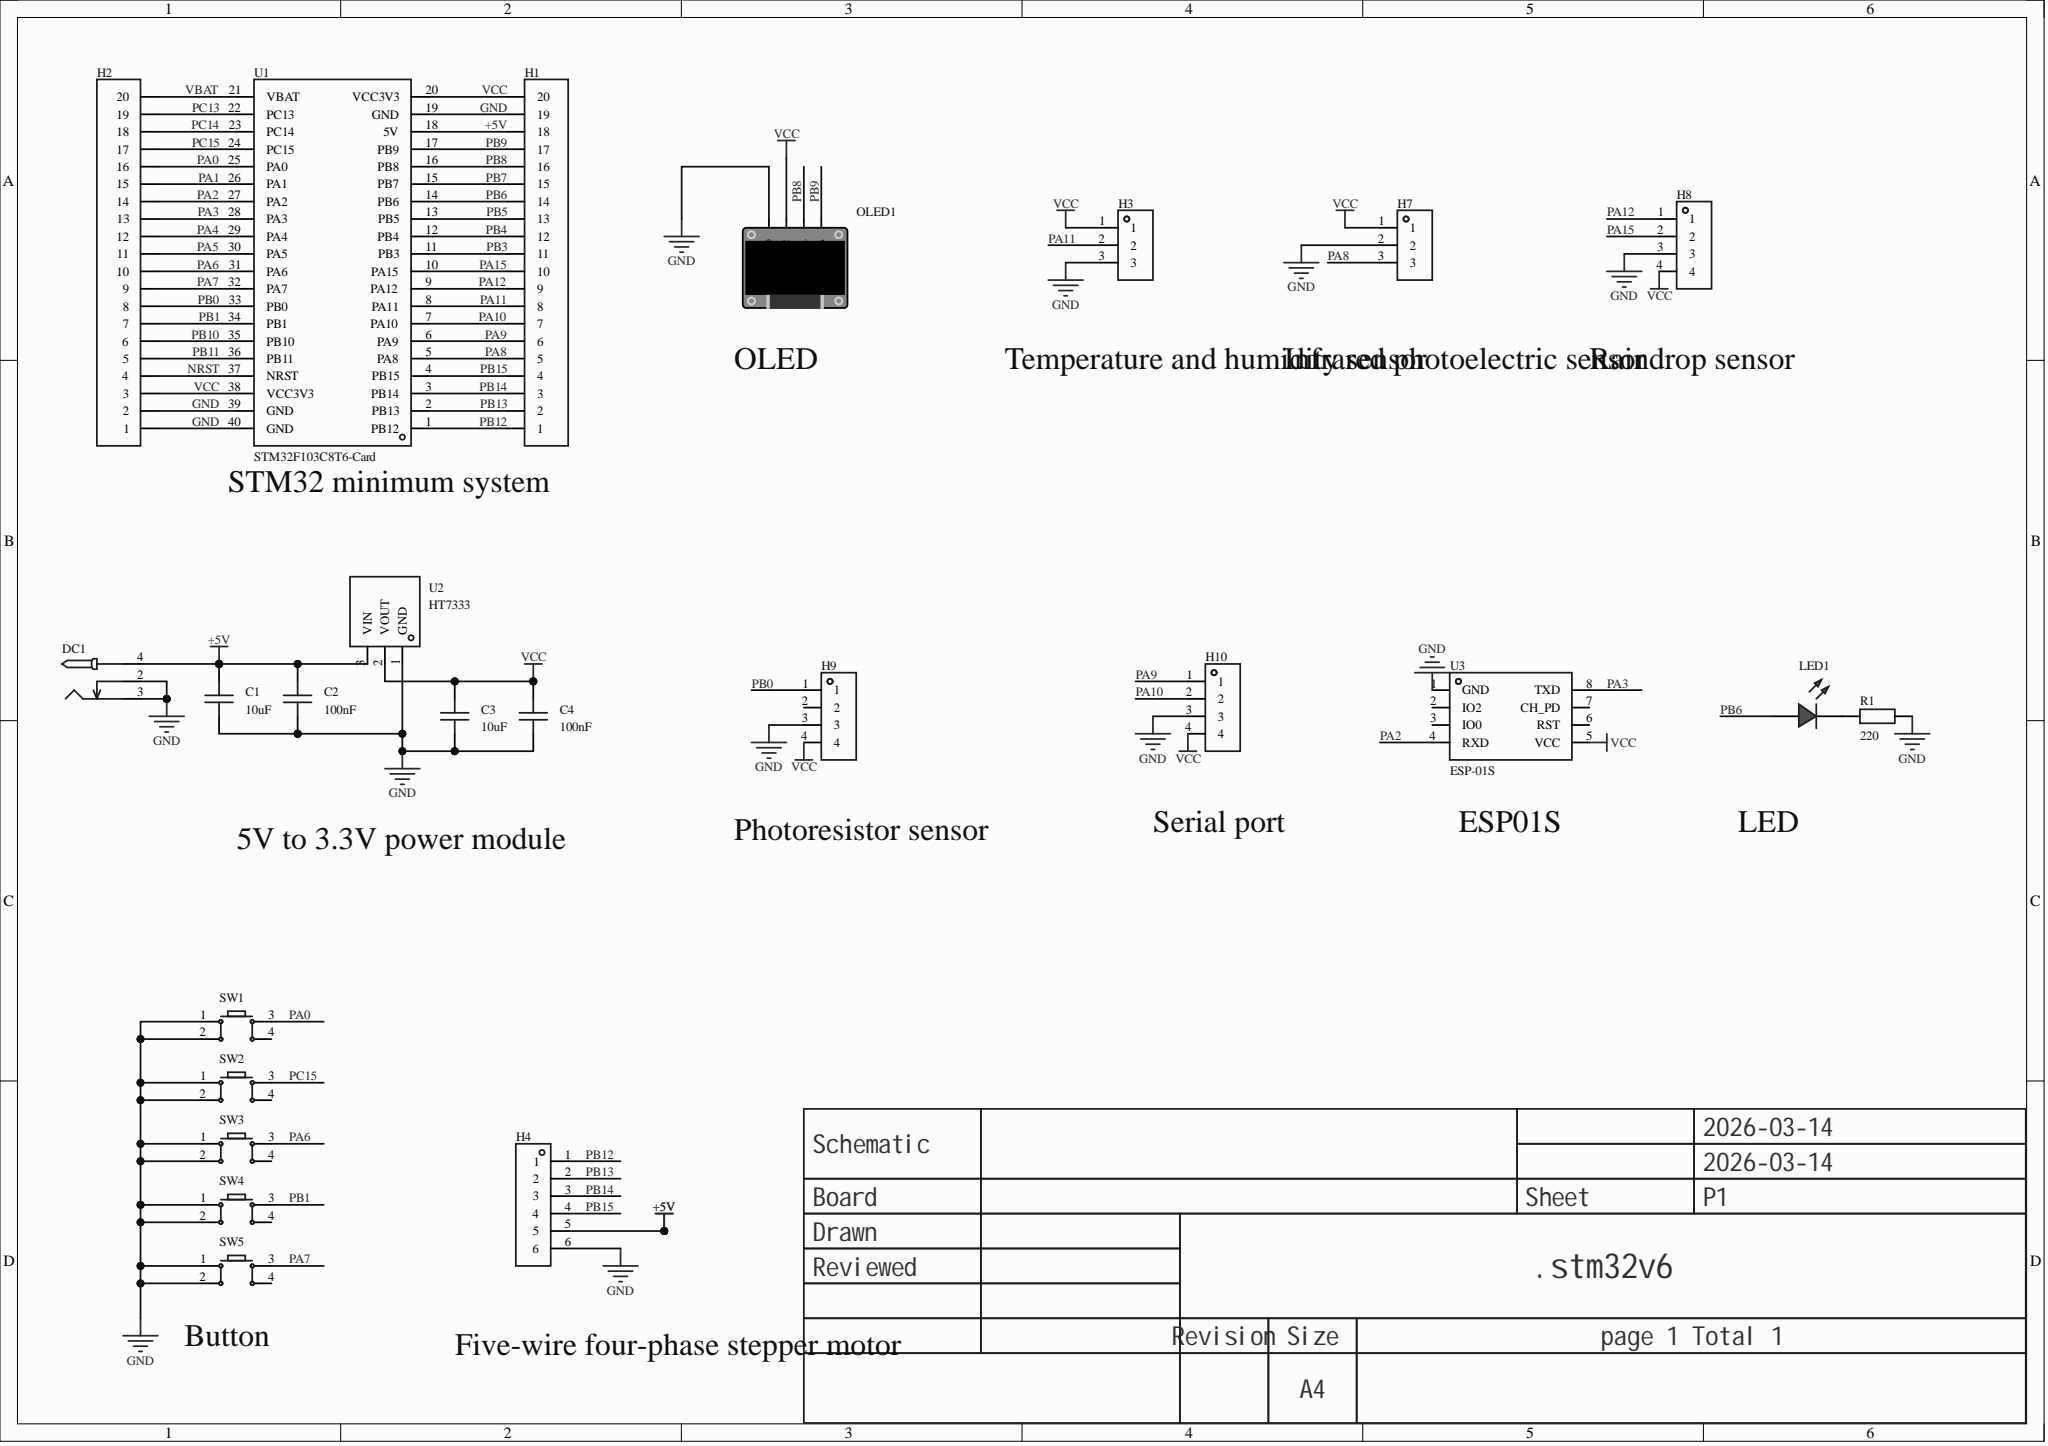Circuit board | Altium Designer | 24 parts | 38 nets
Bill of materials:
Comment,Description,Designator,Footprint,LibRef,Quantity
"10uF","","C1, C3","C0603","CAP_0603","2"
"100nF","","C2, C4","C0603","CAP_0603","2"
"","","DC1","DC-2.0","DC-005_2.0","1"
"","","H1, H2","HDR-TH_20P-P2.54-V-F","HDR-F_2.54_1x20P","2"
"","","H3, H7","HDR-TH_3P-P2.54-V-F","HDR-F_2.54_1x3P","2"
"","","H4","HDR-TH_6P-P2.54-V-F","HDR-F_2.54_1x6P","1"
"","","H8, H9, H10","HDR-TH_4P-P2.54-V-F","HDR-F_2.54_1x4P","3"
"","","LED1","LED_TH-3mm","LED_TH-R_3mm","1"
"","","OLED1","0.96OLED_4P","0.96OLED模块_4P","1"
"220","","R1","Res_1/8W","Res_AXIAL-1/8W","1"
"","","SW1, SW2, SW3, SW4, SW5","SW-TH_4P-L6.0-W6.0-P4.50-LS6.5","Key_TH_6x6x6","5"
"STM32F103C8T6-Card","","U1","CONN-TH_L53.3-W22.9_STM32F103C8T6-CARD","STM32F103C8T6-Card","1"
"HT7333","Output type: fixed; Operating voltage: 12V; Output voltage: 3.3V; Output current: 250mA; Ripple rejection (PSRR): -; Output polarity: positive;","U2","SOT-23-3_L2.9-W1.6-P1.90-LS2.8-BR","HT7333","1"
"ESP-01S","","U3","WIFIM-TH_ESP-01S","ESP-01S_C111009","1"
Netlist (Protel format):
[
C1
C0603
10uF



]
[
C2
C0603
100nF



]
[
C3
C0603
10uF



]
[
C4
C0603
100nF



]
[
DC1
DC-2.0




]
[
H1
HDR-TH_20P-P2.54-V-F




]
[
H2
HDR-TH_20P-P2.54-V-F




]
[
H3
HDR-TH_3P-P2.54-V-F




]
[
H4
HDR-TH_6P-P2.54-V-F




]
[
H7
HDR-TH_3P-P2.54-V-F




]
[
H8
HDR-TH_4P-P2.54-V-F




]
[
H9
HDR-TH_4P-P2.54-V-F




]
[
H10
HDR-TH_4P-P2.54-V-F




]
[
LED1
LED_TH-3mm




]
[
OLED1
0.96OLED_4P




]
[
R1
Res_1/8W
220



]
[
SW1
SW-TH_4P-L6.0-W6.0-P4.50-LS6.5




]
[
SW2
SW-TH_4P-L6.0-W6.0-P4.50-LS6.5




]
[
SW3
SW-TH_4P-L6.0-W6.0-P4.50-LS6.5




]
[
SW4
SW-TH_4P-L6.0-W6.0-P4.50-LS6.5




]
[
SW5
SW-TH_4P-L6.0-W6.0-P4.50-LS6.5




]
[
U1
CONN-TH_L53.3-W22.9_STM32F103C8T6-CARD
STM32F103C8T6-Card



]
[
U2
SOT-23-3_L2.9-W1.6-P1.90-LS2.8-BR
HT7333



]
[
U3
WIFIM-TH_ESP-01S
ESP-01S



]
(
VCC
C3-2
C4-2
H1-20
H2-3
H3-1
H7-1
H8-4
H9-4
H10-4
OLED1-2
U1-20
U1-38
U2-2
U3-5
)
(
VBAT
H2-20
U1-21
)
(
PC15
H2-17
SW2-3
U1-24
)
(
PC14
H2-18
U1-23
)
(
PC13
H2-19
U1-22
)
(
PB15
H1-4
H4-4
U1-4
)
(
PB14
H1-3
H4-3
U1-3
)
(
PB13
H1-2
H4-2
U1-2
)
(
PB12
H1-1
H4-1
U1-1
)
(
PB11
H2-5
U1-36
)
(
PB10
H2-6
U1-35
)
(
PB9
H1-17
OLED1-4
U1-17
)
(
PB8
H1-16
OLED1-3
U1-16
)
(
PB7
H1-15
U1-15
)
(
PB6
H1-14
LED1-1
U1-14
)
(
PB5
H1-13
U1-13
)
(
PB4
H1-12
U1-12
)
(
PB3
H1-11
U1-11
)
(
PB1
H2-7
SW4-3
U1-34
)
(
PB0
H2-8
H9-1
U1-33
)
(
PA15
H1-10
H8-2
U1-10
)
(
PA12
H1-9
H8-1
U1-9
)
(
PA11
H1-8
H3-2
U1-8
)
(
PA10
H1-7
H10-2
U1-7
)
(
PA9
H1-6
H10-1
U1-6
)
(
PA8
H1-5
H7-3
U1-5
)
(
PA7
H2-9
SW5-3
U1-32
)
(
PA6
H2-10
SW3-3
U1-31
)
(
PA5
H2-11
U1-30
)
(
PA4
H2-12
U1-29
)
(
PA3
H2-13
U1-28
U3-8
)
(
PA2
H2-14
U1-27
U3-4
)
(
PA1
H2-15
U1-26
)
(
PA0
H2-16
SW1-3
U1-25
)
(
NRST
H2-4
U1-37
)
(
NetLED1_2
LED1-2
R1-1
)
(
GND
C1-1
C2-1
C3-1
C4-1
DC1-2
DC1-3
H1-19
H2-1
H2-2
H3-3
H4-6
H7-2
H8-3
H9-3
H10-3
OLED1-1
R1-2
SW1-1
SW1-2
SW2-1
SW2-2
SW3-1
SW3-2
SW4-1
SW4-2
SW5-1
SW5-2
U1-19
U1-39
U1-40
U2-1
U3-1
)
(
+5V
C1-2
C2-2
DC1-4
H1-18
H4-5
U1-18
U2-3
)